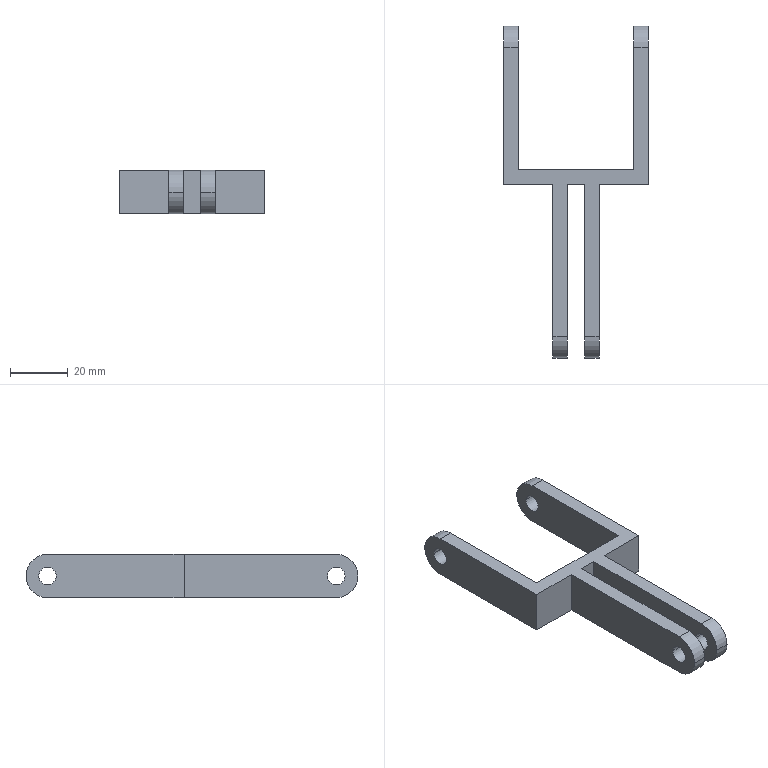Part | SolidWorks | features Extrusion 1, ICE 1 | 1 solid | 28 faces | box 50 x 115 x 15 mm | volume 19202 mm3 | cylinder 14 | plane 14 | commonest cylinder face diameters 6 x8 15 x6
STEP:
#1=CARTESIAN_POINT('',(8.,15.272,7.5));
#2=VERTEX_POINT('',#1);
#3=CARTESIAN_POINT('',(8.,9.272,7.5));
#4=VERTEX_POINT('',#3);
#5=CARTESIAN_POINT('',(8.,12.272,7.5));
#6=DIRECTION('',(-1.,0.,0.));
#7=DIRECTION('',(0.,-1.,0.));
#8=AXIS2_PLACEMENT_3D('',#5,#6,#7);
#9=CIRCLE('',#8,3.);
#10=EDGE_CURVE('',#2,#4,#9,.T.);
#11=ORIENTED_EDGE('',*,*,#10,.F.);
#12=CARTESIAN_POINT('',(3.,15.272,7.5));
#13=VERTEX_POINT('',#12);
#14=CARTESIAN_POINT('',(25.,15.272,7.5));
#15=DIRECTION('',(-1.,0.,0.));
#16=VECTOR('',#15,1000.);
#17=LINE('',#14,#16);
#18=EDGE_CURVE('',#2,#13,#17,.T.);
#19=ORIENTED_EDGE('',*,*,#18,.T.);
#20=CARTESIAN_POINT('',(3.,9.272,7.5));
#21=VERTEX_POINT('',#20);
#22=CARTESIAN_POINT('',(3.,12.272,7.5));
#23=DIRECTION('',(1.,0.,0.));
#24=DIRECTION('',(0.,1.,0.));
#25=AXIS2_PLACEMENT_3D('',#22,#23,#24);
#26=CIRCLE('',#25,3.);
#27=EDGE_CURVE('',#21,#13,#26,.T.);
#28=ORIENTED_EDGE('',*,*,#27,.F.);
#29=CARTESIAN_POINT('',(25.,9.272,7.5));
#30=DIRECTION('',(-1.,0.,0.));
#31=VECTOR('',#30,1000.);
#32=LINE('',#29,#31);
#33=EDGE_CURVE('',#4,#21,#32,.T.);
#34=ORIENTED_EDGE('',*,*,#33,.F.);
#35=EDGE_LOOP('',(#11,#19,#28,#34));
#36=FACE_OUTER_BOUND('',#35,.T.);
#37=CARTESIAN_POINT('',(25.,12.272,7.5));
#38=DIRECTION('',(-1.,0.,0.));
#39=DIRECTION('',(0.,-1.,0.));
#40=AXIS2_PLACEMENT_3D('',#37,#38,#39);
#41=CYLINDRICAL_SURFACE('',#40,3.);
#42=ADVANCED_FACE('',(#36),#41,.F.);
#43=CARTESIAN_POINT('',(25.,115.272,7.5));
#44=VERTEX_POINT('',#43);
#45=CARTESIAN_POINT('',(25.,109.272,7.5));
#46=VERTEX_POINT('',#45);
#47=CARTESIAN_POINT('',(25.,112.272,7.5));
#48=DIRECTION('',(-1.,0.,0.));
#49=DIRECTION('',(0.,-1.,0.));
#50=AXIS2_PLACEMENT_3D('',#47,#48,#49);
#51=CIRCLE('',#50,3.);
#52=EDGE_CURVE('',#44,#46,#51,.T.);
#53=ORIENTED_EDGE('',*,*,#52,.F.);
#54=CARTESIAN_POINT('',(20.,115.272,7.5));
#55=VERTEX_POINT('',#54);
#56=CARTESIAN_POINT('',(25.,115.272,7.5));
#57=DIRECTION('',(-1.,0.,0.));
#58=VECTOR('',#57,1000.);
#59=LINE('',#56,#58);
#60=EDGE_CURVE('',#44,#55,#59,.T.);
#61=ORIENTED_EDGE('',*,*,#60,.T.);
#62=CARTESIAN_POINT('',(20.,109.272,7.5));
#63=VERTEX_POINT('',#62);
#64=CARTESIAN_POINT('',(20.,112.272,7.5));
#65=DIRECTION('',(1.,0.,0.));
#66=DIRECTION('',(0.,0.,-1.));
#67=AXIS2_PLACEMENT_3D('',#64,#65,#66);
#68=CIRCLE('',#67,3.);
#69=EDGE_CURVE('',#63,#55,#68,.T.);
#70=ORIENTED_EDGE('',*,*,#69,.F.);
#71=CARTESIAN_POINT('',(25.,109.272,7.5));
#72=DIRECTION('',(-1.,0.,0.));
#73=VECTOR('',#72,1000.);
#74=LINE('',#71,#73);
#75=EDGE_CURVE('',#46,#63,#74,.T.);
#76=ORIENTED_EDGE('',*,*,#75,.F.);
#77=EDGE_LOOP('',(#53,#61,#70,#76));
#78=FACE_OUTER_BOUND('',#77,.T.);
#79=CARTESIAN_POINT('',(25.,112.272,7.5));
#80=DIRECTION('',(-1.,0.,0.));
#81=DIRECTION('',(0.,-1.,0.));
#82=AXIS2_PLACEMENT_3D('',#79,#80,#81);
#83=CYLINDRICAL_SURFACE('',#82,3.);
#84=ADVANCED_FACE('',(#78),#83,.F.);
#85=CARTESIAN_POINT('',(-20.,115.272,7.5));
#86=VERTEX_POINT('',#85);
#87=CARTESIAN_POINT('',(-20.,109.272,7.5));
#88=VERTEX_POINT('',#87);
#89=CARTESIAN_POINT('',(-20.,112.272,7.5));
#90=DIRECTION('',(-1.,0.,0.));
#91=DIRECTION('',(0.,0.,1.));
#92=AXIS2_PLACEMENT_3D('',#89,#90,#91);
#93=CIRCLE('',#92,3.);
#94=EDGE_CURVE('',#86,#88,#93,.T.);
#95=ORIENTED_EDGE('',*,*,#94,.F.);
#96=CARTESIAN_POINT('',(-25.,115.272,7.5));
#97=VERTEX_POINT('',#96);
#98=CARTESIAN_POINT('',(25.,115.272,7.5));
#99=DIRECTION('',(-1.,0.,0.));
#100=VECTOR('',#99,1000.);
#101=LINE('',#98,#100);
#102=EDGE_CURVE('',#86,#97,#101,.T.);
#103=ORIENTED_EDGE('',*,*,#102,.T.);
#104=CARTESIAN_POINT('',(-25.,109.272,7.5));
#105=VERTEX_POINT('',#104);
#106=CARTESIAN_POINT('',(-25.,112.272,7.5));
#107=DIRECTION('',(-1.,0.,0.));
#108=DIRECTION('',(0.,-1.,0.));
#109=AXIS2_PLACEMENT_3D('',#106,#107,#108);
#110=CIRCLE('',#109,3.);
#111=EDGE_CURVE('',#97,#105,#110,.T.);
#112=ORIENTED_EDGE('',*,*,#111,.T.);
#113=CARTESIAN_POINT('',(25.,109.272,7.5));
#114=DIRECTION('',(-1.,0.,0.));
#115=VECTOR('',#114,1000.);
#116=LINE('',#113,#115);
#117=EDGE_CURVE('',#88,#105,#116,.T.);
#118=ORIENTED_EDGE('',*,*,#117,.F.);
#119=EDGE_LOOP('',(#95,#103,#112,#118));
#120=FACE_OUTER_BOUND('',#119,.T.);
#121=CARTESIAN_POINT('',(25.,112.272,7.5));
#122=DIRECTION('',(-1.,0.,0.));
#123=DIRECTION('',(0.,-1.,0.));
#124=AXIS2_PLACEMENT_3D('',#121,#122,#123);
#125=CYLINDRICAL_SURFACE('',#124,3.);
#126=ADVANCED_FACE('',(#120),#125,.F.);
#127=CARTESIAN_POINT('',(-3.,15.272,7.5));
#128=VERTEX_POINT('',#127);
#129=CARTESIAN_POINT('',(-3.,9.272,7.5));
#130=VERTEX_POINT('',#129);
#131=CARTESIAN_POINT('',(-3.,12.272,7.5));
#132=DIRECTION('',(-1.,0.,0.));
#133=DIRECTION('',(0.,-1.,0.));
#134=AXIS2_PLACEMENT_3D('',#131,#132,#133);
#135=CIRCLE('',#134,3.);
#136=EDGE_CURVE('',#128,#130,#135,.T.);
#137=ORIENTED_EDGE('',*,*,#136,.F.);
#138=CARTESIAN_POINT('',(-8.,15.272,7.5));
#139=VERTEX_POINT('',#138);
#140=CARTESIAN_POINT('',(25.,15.272,7.5));
#141=DIRECTION('',(-1.,0.,0.));
#142=VECTOR('',#141,1000.);
#143=LINE('',#140,#142);
#144=EDGE_CURVE('',#128,#139,#143,.T.);
#145=ORIENTED_EDGE('',*,*,#144,.T.);
#146=CARTESIAN_POINT('',(-8.,9.272,7.5));
#147=VERTEX_POINT('',#146);
#148=CARTESIAN_POINT('',(-8.,12.272,7.5));
#149=DIRECTION('',(1.,0.,0.));
#150=DIRECTION('',(0.,1.,0.));
#151=AXIS2_PLACEMENT_3D('',#148,#149,#150);
#152=CIRCLE('',#151,3.);
#153=EDGE_CURVE('',#147,#139,#152,.T.);
#154=ORIENTED_EDGE('',*,*,#153,.F.);
#155=CARTESIAN_POINT('',(25.,9.272,7.5));
#156=DIRECTION('',(-1.,0.,0.));
#157=VECTOR('',#156,1000.);
#158=LINE('',#155,#157);
#159=EDGE_CURVE('',#130,#147,#158,.T.);
#160=ORIENTED_EDGE('',*,*,#159,.F.);
#161=EDGE_LOOP('',(#137,#145,#154,#160));
#162=FACE_OUTER_BOUND('',#161,.T.);
#163=CARTESIAN_POINT('',(25.,12.272,7.5));
#164=DIRECTION('',(-1.,0.,0.));
#165=DIRECTION('',(0.,-1.,0.));
#166=AXIS2_PLACEMENT_3D('',#163,#164,#165);
#167=CYLINDRICAL_SURFACE('',#166,3.);
#168=ADVANCED_FACE('',(#162),#167,.F.);
#169=CARTESIAN_POINT('',(8.,4.772,7.5));
#170=VERTEX_POINT('',#169);
#171=CARTESIAN_POINT('',(8.,12.272,0.));
#172=VERTEX_POINT('',#171);
#173=CARTESIAN_POINT('',(8.,12.272,7.5));
#174=DIRECTION('',(1.,0.,0.));
#175=DIRECTION('',(0.,-1.,0.));
#176=AXIS2_PLACEMENT_3D('',#173,#174,#175);
#177=CIRCLE('',#176,7.5);
#178=EDGE_CURVE('',#170,#172,#177,.T.);
#179=ORIENTED_EDGE('',*,*,#178,.F.);
#180=CARTESIAN_POINT('',(3.,4.772,7.5));
#181=VERTEX_POINT('',#180);
#182=CARTESIAN_POINT('',(25.,4.772,7.5));
#183=DIRECTION('',(-1.,0.,0.));
#184=VECTOR('',#183,1000.);
#185=LINE('',#182,#184);
#186=EDGE_CURVE('',#170,#181,#185,.T.);
#187=ORIENTED_EDGE('',*,*,#186,.T.);
#188=CARTESIAN_POINT('',(3.,12.272,0.));
#189=VERTEX_POINT('',#188);
#190=CARTESIAN_POINT('',(3.,12.272,7.5));
#191=DIRECTION('',(-1.,0.,0.));
#192=DIRECTION('',(0.,1.,0.));
#193=AXIS2_PLACEMENT_3D('',#190,#191,#192);
#194=CIRCLE('',#193,7.5);
#195=EDGE_CURVE('',#189,#181,#194,.T.);
#196=ORIENTED_EDGE('',*,*,#195,.F.);
#197=CARTESIAN_POINT('',(0.,12.272,0.));
#198=DIRECTION('',(-1.,0.,0.));
#199=VECTOR('',#198,1000.);
#200=LINE('',#197,#199);
#201=EDGE_CURVE('',#172,#189,#200,.T.);
#202=ORIENTED_EDGE('',*,*,#201,.F.);
#203=EDGE_LOOP('',(#179,#187,#196,#202));
#204=FACE_OUTER_BOUND('',#203,.T.);
#205=CARTESIAN_POINT('',(25.,12.272,7.5));
#206=DIRECTION('',(-1.,0.,0.));
#207=DIRECTION('',(0.,-1.,0.));
#208=AXIS2_PLACEMENT_3D('',#205,#206,#207);
#209=CYLINDRICAL_SURFACE('',#208,7.5);
#210=ADVANCED_FACE('',(#204),#209,.T.);
#211=CARTESIAN_POINT('',(-3.,4.772,7.5));
#212=VERTEX_POINT('',#211);
#213=CARTESIAN_POINT('',(-3.,12.272,0.));
#214=VERTEX_POINT('',#213);
#215=CARTESIAN_POINT('',(-3.,12.272,7.5));
#216=DIRECTION('',(1.,0.,0.));
#217=DIRECTION('',(0.,-1.,0.));
#218=AXIS2_PLACEMENT_3D('',#215,#216,#217);
#219=CIRCLE('',#218,7.5);
#220=EDGE_CURVE('',#212,#214,#219,.T.);
#221=ORIENTED_EDGE('',*,*,#220,.F.);
#222=CARTESIAN_POINT('',(-8.,4.772,7.5));
#223=VERTEX_POINT('',#222);
#224=CARTESIAN_POINT('',(25.,4.772,7.5));
#225=DIRECTION('',(-1.,0.,0.));
#226=VECTOR('',#225,1000.);
#227=LINE('',#224,#226);
#228=EDGE_CURVE('',#212,#223,#227,.T.);
#229=ORIENTED_EDGE('',*,*,#228,.T.);
#230=CARTESIAN_POINT('',(-8.,12.272,0.));
#231=VERTEX_POINT('',#230);
#232=CARTESIAN_POINT('',(-8.,12.272,7.5));
#233=DIRECTION('',(-1.,0.,0.));
#234=DIRECTION('',(0.,1.,0.));
#235=AXIS2_PLACEMENT_3D('',#232,#233,#234);
#236=CIRCLE('',#235,7.5);
#237=EDGE_CURVE('',#231,#223,#236,.T.);
#238=ORIENTED_EDGE('',*,*,#237,.F.);
#239=CARTESIAN_POINT('',(0.,12.272,0.));
#240=DIRECTION('',(-1.,0.,0.));
#241=VECTOR('',#240,1000.);
#242=LINE('',#239,#241);
#243=EDGE_CURVE('',#214,#231,#242,.T.);
#244=ORIENTED_EDGE('',*,*,#243,.F.);
#245=EDGE_LOOP('',(#221,#229,#238,#244));
#246=FACE_OUTER_BOUND('',#245,.T.);
#247=CARTESIAN_POINT('',(25.,12.272,7.5));
#248=DIRECTION('',(-1.,0.,0.));
#249=DIRECTION('',(0.,-1.,0.));
#250=AXIS2_PLACEMENT_3D('',#247,#248,#249);
#251=CYLINDRICAL_SURFACE('',#250,7.5);
#252=ADVANCED_FACE('',(#246),#251,.T.);
#253=CARTESIAN_POINT('',(-3.,12.272,15.));
#254=VERTEX_POINT('',#253);
#255=CARTESIAN_POINT('',(-3.,65.,15.));
#256=VERTEX_POINT('',#255);
#257=CARTESIAN_POINT('',(-3.,0.,15.));
#258=DIRECTION('',(0.,1.,0.));
#259=VECTOR('',#258,1000.);
#260=LINE('',#257,#259);
#261=EDGE_CURVE('',#254,#256,#260,.T.);
#262=ORIENTED_EDGE('',*,*,#261,.F.);
#263=CARTESIAN_POINT('',(-3.,12.272,7.5));
#264=DIRECTION('',(1.,0.,0.));
#265=DIRECTION('',(0.,-1.,0.));
#266=AXIS2_PLACEMENT_3D('',#263,#264,#265);
#267=CIRCLE('',#266,7.5);
#268=EDGE_CURVE('',#254,#212,#267,.T.);
#269=ORIENTED_EDGE('',*,*,#268,.T.);
#270=ORIENTED_EDGE('',*,*,#220,.T.);
#271=CARTESIAN_POINT('',(-3.,65.,0.));
#272=VERTEX_POINT('',#271);
#273=CARTESIAN_POINT('',(-3.,0.,0.));
#274=DIRECTION('',(0.,1.,0.));
#275=VECTOR('',#274,1000.);
#276=LINE('',#273,#275);
#277=EDGE_CURVE('',#214,#272,#276,.T.);
#278=ORIENTED_EDGE('',*,*,#277,.T.);
#279=CARTESIAN_POINT('',(-3.,65.,15.));
#280=DIRECTION('',(0.,0.,-1.));
#281=VECTOR('',#280,1000.);
#282=LINE('',#279,#281);
#283=EDGE_CURVE('',#256,#272,#282,.T.);
#284=ORIENTED_EDGE('',*,*,#283,.F.);
#285=EDGE_LOOP('',(#262,#269,#270,#278,#284));
#286=FACE_OUTER_BOUND('',#285,.T.);
#287=CARTESIAN_POINT('',(-3.,12.272,7.5));
#288=DIRECTION('',(-1.,0.,0.));
#289=DIRECTION('',(0.,-1.,0.));
#290=AXIS2_PLACEMENT_3D('',#287,#288,#289);
#291=CIRCLE('',#290,3.);
#292=EDGE_CURVE('',#130,#128,#291,.T.);
#293=ORIENTED_EDGE('',*,*,#292,.T.);
#294=ORIENTED_EDGE('',*,*,#136,.T.);
#295=EDGE_LOOP('',(#293,#294));
#296=FACE_BOUND('',#295,.T.);
#297=CARTESIAN_POINT('',(-3.,0.,15.));
#298=DIRECTION('',(-1.,0.,0.));
#299=DIRECTION('',(0.,-1.,0.));
#300=AXIS2_PLACEMENT_3D('',#297,#298,#299);
#301=PLANE('',#300);
#302=ADVANCED_FACE('',(#286,#296),#301,.F.);
#303=CARTESIAN_POINT('',(3.,65.,0.));
#304=VERTEX_POINT('',#303);
#305=CARTESIAN_POINT('',(3.,0.,0.));
#306=DIRECTION('',(0.,-1.,0.));
#307=VECTOR('',#306,1000.);
#308=LINE('',#305,#307);
#309=EDGE_CURVE('',#304,#189,#308,.T.);
#310=ORIENTED_EDGE('',*,*,#309,.T.);
#311=ORIENTED_EDGE('',*,*,#195,.T.);
#312=CARTESIAN_POINT('',(3.,12.272,15.));
#313=VERTEX_POINT('',#312);
#314=CARTESIAN_POINT('',(3.,12.272,7.5));
#315=DIRECTION('',(-1.,0.,0.));
#316=DIRECTION('',(0.,1.,0.));
#317=AXIS2_PLACEMENT_3D('',#314,#315,#316);
#318=CIRCLE('',#317,7.5);
#319=EDGE_CURVE('',#181,#313,#318,.T.);
#320=ORIENTED_EDGE('',*,*,#319,.T.);
#321=CARTESIAN_POINT('',(3.,65.,15.));
#322=VERTEX_POINT('',#321);
#323=CARTESIAN_POINT('',(3.,0.,15.));
#324=DIRECTION('',(0.,-1.,0.));
#325=VECTOR('',#324,1000.);
#326=LINE('',#323,#325);
#327=EDGE_CURVE('',#322,#313,#326,.T.);
#328=ORIENTED_EDGE('',*,*,#327,.F.);
#329=CARTESIAN_POINT('',(3.,65.,15.));
#330=DIRECTION('',(0.,0.,-1.));
#331=VECTOR('',#330,1000.);
#332=LINE('',#329,#331);
#333=EDGE_CURVE('',#322,#304,#332,.T.);
#334=ORIENTED_EDGE('',*,*,#333,.T.);
#335=EDGE_LOOP('',(#310,#311,#320,#328,#334));
#336=FACE_OUTER_BOUND('',#335,.T.);
#337=ORIENTED_EDGE('',*,*,#27,.T.);
#338=CARTESIAN_POINT('',(3.,12.272,7.5));
#339=DIRECTION('',(1.,0.,0.));
#340=DIRECTION('',(0.,1.,0.));
#341=AXIS2_PLACEMENT_3D('',#338,#339,#340);
#342=CIRCLE('',#341,3.);
#343=EDGE_CURVE('',#13,#21,#342,.T.);
#344=ORIENTED_EDGE('',*,*,#343,.T.);
#345=EDGE_LOOP('',(#337,#344));
#346=FACE_BOUND('',#345,.T.);
#347=CARTESIAN_POINT('',(3.,0.,15.));
#348=DIRECTION('',(1.,0.,0.));
#349=DIRECTION('',(0.,1.,0.));
#350=AXIS2_PLACEMENT_3D('',#347,#348,#349);
#351=PLANE('',#350);
#352=ADVANCED_FACE('',(#336,#346),#351,.F.);
#353=CARTESIAN_POINT('',(8.,12.272,15.));
#354=VERTEX_POINT('',#353);
#355=CARTESIAN_POINT('',(8.,65.,15.));
#356=VERTEX_POINT('',#355);
#357=CARTESIAN_POINT('',(8.,65.,15.));
#358=DIRECTION('',(0.,1.,0.));
#359=VECTOR('',#358,1000.);
#360=LINE('',#357,#359);
#361=EDGE_CURVE('',#354,#356,#360,.T.);
#362=ORIENTED_EDGE('',*,*,#361,.F.);
#363=CARTESIAN_POINT('',(8.,12.272,7.5));
#364=DIRECTION('',(1.,0.,0.));
#365=DIRECTION('',(0.,-1.,0.));
#366=AXIS2_PLACEMENT_3D('',#363,#364,#365);
#367=CIRCLE('',#366,7.5);
#368=EDGE_CURVE('',#354,#170,#367,.T.);
#369=ORIENTED_EDGE('',*,*,#368,.T.);
#370=ORIENTED_EDGE('',*,*,#178,.T.);
#371=CARTESIAN_POINT('',(8.,65.,0.));
#372=VERTEX_POINT('',#371);
#373=CARTESIAN_POINT('',(8.,65.,0.));
#374=DIRECTION('',(0.,1.,0.));
#375=VECTOR('',#374,1000.);
#376=LINE('',#373,#375);
#377=EDGE_CURVE('',#172,#372,#376,.T.);
#378=ORIENTED_EDGE('',*,*,#377,.T.);
#379=CARTESIAN_POINT('',(8.,65.,15.));
#380=DIRECTION('',(0.,0.,-1.));
#381=VECTOR('',#380,1000.);
#382=LINE('',#379,#381);
#383=EDGE_CURVE('',#356,#372,#382,.T.);
#384=ORIENTED_EDGE('',*,*,#383,.F.);
#385=EDGE_LOOP('',(#362,#369,#370,#378,#384));
#386=FACE_OUTER_BOUND('',#385,.T.);
#387=CARTESIAN_POINT('',(8.,12.272,7.5));
#388=DIRECTION('',(-1.,0.,0.));
#389=DIRECTION('',(0.,-1.,0.));
#390=AXIS2_PLACEMENT_3D('',#387,#388,#389);
#391=CIRCLE('',#390,3.);
#392=EDGE_CURVE('',#4,#2,#391,.T.);
#393=ORIENTED_EDGE('',*,*,#392,.T.);
#394=ORIENTED_EDGE('',*,*,#10,.T.);
#395=EDGE_LOOP('',(#393,#394));
#396=FACE_BOUND('',#395,.T.);
#397=CARTESIAN_POINT('',(8.,65.,15.));
#398=DIRECTION('',(-1.,0.,0.));
#399=DIRECTION('',(0.,-1.,0.));
#400=AXIS2_PLACEMENT_3D('',#397,#398,#399);
#401=PLANE('',#400);
#402=ADVANCED_FACE('',(#386,#396),#401,.F.);
#403=CARTESIAN_POINT('',(-8.,65.,0.));
#404=VERTEX_POINT('',#403);
#405=CARTESIAN_POINT('',(-8.,65.,0.));
#406=DIRECTION('',(0.,-1.,0.));
#407=VECTOR('',#406,1000.);
#408=LINE('',#405,#407);
#409=EDGE_CURVE('',#404,#231,#408,.T.);
#410=ORIENTED_EDGE('',*,*,#409,.T.);
#411=ORIENTED_EDGE('',*,*,#237,.T.);
#412=CARTESIAN_POINT('',(-8.,12.272,15.));
#413=VERTEX_POINT('',#412);
#414=CARTESIAN_POINT('',(-8.,12.272,7.5));
#415=DIRECTION('',(-1.,0.,0.));
#416=DIRECTION('',(0.,1.,0.));
#417=AXIS2_PLACEMENT_3D('',#414,#415,#416);
#418=CIRCLE('',#417,7.5);
#419=EDGE_CURVE('',#223,#413,#418,.T.);
#420=ORIENTED_EDGE('',*,*,#419,.T.);
#421=CARTESIAN_POINT('',(-8.,65.,15.));
#422=VERTEX_POINT('',#421);
#423=CARTESIAN_POINT('',(-8.,65.,15.));
#424=DIRECTION('',(0.,-1.,0.));
#425=VECTOR('',#424,1000.);
#426=LINE('',#423,#425);
#427=EDGE_CURVE('',#422,#413,#426,.T.);
#428=ORIENTED_EDGE('',*,*,#427,.F.);
#429=CARTESIAN_POINT('',(-8.,65.,15.));
#430=DIRECTION('',(0.,0.,-1.));
#431=VECTOR('',#430,1000.);
#432=LINE('',#429,#431);
#433=EDGE_CURVE('',#422,#404,#432,.T.);
#434=ORIENTED_EDGE('',*,*,#433,.T.);
#435=EDGE_LOOP('',(#410,#411,#420,#428,#434));
#436=FACE_OUTER_BOUND('',#435,.T.);
#437=ORIENTED_EDGE('',*,*,#153,.T.);
#438=CARTESIAN_POINT('',(-8.,12.272,7.5));
#439=DIRECTION('',(1.,0.,0.));
#440=DIRECTION('',(0.,1.,0.));
#441=AXIS2_PLACEMENT_3D('',#438,#439,#440);
#442=CIRCLE('',#441,3.);
#443=EDGE_CURVE('',#139,#147,#442,.T.);
#444=ORIENTED_EDGE('',*,*,#443,.T.);
#445=EDGE_LOOP('',(#437,#444));
#446=FACE_BOUND('',#445,.T.);
#447=CARTESIAN_POINT('',(-8.,65.,15.));
#448=DIRECTION('',(1.,0.,0.));
#449=DIRECTION('',(0.,1.,0.));
#450=AXIS2_PLACEMENT_3D('',#447,#448,#449);
#451=PLANE('',#450);
#452=ADVANCED_FACE('',(#436,#446),#451,.F.);
#453=CARTESIAN_POINT('',(-3.,65.,0.));
#454=DIRECTION('',(1.,0.,0.));
#455=VECTOR('',#454,1000.);
#456=LINE('',#453,#455);
#457=EDGE_CURVE('',#272,#304,#456,.T.);
#458=ORIENTED_EDGE('',*,*,#457,.T.);
#459=ORIENTED_EDGE('',*,*,#333,.F.);
#460=CARTESIAN_POINT('',(-3.,65.,15.));
#461=DIRECTION('',(1.,0.,0.));
#462=VECTOR('',#461,1000.);
#463=LINE('',#460,#462);
#464=EDGE_CURVE('',#256,#322,#463,.T.);
#465=ORIENTED_EDGE('',*,*,#464,.F.);
#466=ORIENTED_EDGE('',*,*,#283,.T.);
#467=EDGE_LOOP('',(#458,#459,#465,#466));
#468=FACE_OUTER_BOUND('',#467,.T.);
#469=CARTESIAN_POINT('',(-3.,65.,15.));
#470=DIRECTION('',(0.,1.,0.));
#471=DIRECTION('',(0.,0.,1.));
#472=AXIS2_PLACEMENT_3D('',#469,#470,#471);
#473=PLANE('',#472);
#474=ADVANCED_FACE('',(#468),#473,.F.);
#475=CARTESIAN_POINT('',(25.,65.,0.));
#476=VERTEX_POINT('',#475);
#477=CARTESIAN_POINT('',(25.,65.,0.));
#478=DIRECTION('',(1.,0.,0.));
#479=VECTOR('',#478,1000.);
#480=LINE('',#477,#479);
#481=EDGE_CURVE('',#372,#476,#480,.T.);
#482=ORIENTED_EDGE('',*,*,#481,.T.);
#483=CARTESIAN_POINT('',(25.,65.,15.));
#484=VERTEX_POINT('',#483);
#485=CARTESIAN_POINT('',(25.,65.,15.));
#486=DIRECTION('',(0.,0.,-1.));
#487=VECTOR('',#486,1000.);
#488=LINE('',#485,#487);
#489=EDGE_CURVE('',#484,#476,#488,.T.);
#490=ORIENTED_EDGE('',*,*,#489,.F.);
#491=CARTESIAN_POINT('',(25.,65.,15.));
#492=DIRECTION('',(1.,0.,0.));
#493=VECTOR('',#492,1000.);
#494=LINE('',#491,#493);
#495=EDGE_CURVE('',#356,#484,#494,.T.);
#496=ORIENTED_EDGE('',*,*,#495,.F.);
#497=ORIENTED_EDGE('',*,*,#383,.T.);
#498=EDGE_LOOP('',(#482,#490,#496,#497));
#499=FACE_OUTER_BOUND('',#498,.T.);
#500=CARTESIAN_POINT('',(25.,65.,15.));
#501=DIRECTION('',(0.,1.,0.));
#502=DIRECTION('',(0.,0.,1.));
#503=AXIS2_PLACEMENT_3D('',#500,#501,#502);
#504=PLANE('',#503);
#505=ADVANCED_FACE('',(#499),#504,.F.);
#506=CARTESIAN_POINT('',(25.,112.272,7.5));
#507=DIRECTION('',(-1.,0.,0.));
#508=DIRECTION('',(0.,-1.,0.));
#509=AXIS2_PLACEMENT_3D('',#506,#507,#508);
#510=CIRCLE('',#509,3.);
#511=EDGE_CURVE('',#46,#44,#510,.T.);
#512=ORIENTED_EDGE('',*,*,#511,.T.);
#513=ORIENTED_EDGE('',*,*,#52,.T.);
#514=EDGE_LOOP('',(#512,#513));
#515=FACE_BOUND('',#514,.T.);
#516=CARTESIAN_POINT('',(25.,112.272,0.));
#517=VERTEX_POINT('',#516);
#518=CARTESIAN_POINT('',(25.,120.,0.));
#519=DIRECTION('',(0.,1.,0.));
#520=VECTOR('',#519,1000.);
#521=LINE('',#518,#520);
#522=EDGE_CURVE('',#476,#517,#521,.T.);
#523=ORIENTED_EDGE('',*,*,#522,.T.);
#524=CARTESIAN_POINT('',(25.,112.272,15.));
#525=VERTEX_POINT('',#524);
#526=CARTESIAN_POINT('',(25.,112.272,7.5));
#527=DIRECTION('',(1.,0.,0.));
#528=DIRECTION('',(0.,-1.,0.));
#529=AXIS2_PLACEMENT_3D('',#526,#527,#528);
#530=CIRCLE('',#529,7.5);
#531=EDGE_CURVE('',#517,#525,#530,.T.);
#532=ORIENTED_EDGE('',*,*,#531,.T.);
#533=CARTESIAN_POINT('',(25.,120.,15.));
#534=DIRECTION('',(0.,1.,0.));
#535=VECTOR('',#534,1000.);
#536=LINE('',#533,#535);
#537=EDGE_CURVE('',#484,#525,#536,.T.);
#538=ORIENTED_EDGE('',*,*,#537,.F.);
#539=ORIENTED_EDGE('',*,*,#489,.T.);
#540=EDGE_LOOP('',(#523,#532,#538,#539));
#541=FACE_OUTER_BOUND('',#540,.T.);
#542=CARTESIAN_POINT('',(25.,120.,15.));
#543=DIRECTION('',(-1.,0.,0.));
#544=DIRECTION('',(0.,-1.,0.));
#545=AXIS2_PLACEMENT_3D('',#542,#543,#544);
#546=PLANE('',#545);
#547=ADVANCED_FACE('',(#515,#541),#546,.F.);
#548=ORIENTED_EDGE('',*,*,#69,.T.);
#549=CARTESIAN_POINT('',(20.,112.272,7.5));
#550=DIRECTION('',(1.,0.,0.));
#551=DIRECTION('',(0.,0.,-1.));
#552=AXIS2_PLACEMENT_3D('',#549,#550,#551);
#553=CIRCLE('',#552,3.);
#554=EDGE_CURVE('',#55,#63,#553,.T.);
#555=ORIENTED_EDGE('',*,*,#554,.T.);
#556=EDGE_LOOP('',(#548,#555));
#557=FACE_BOUND('',#556,.T.);
#558=CARTESIAN_POINT('',(20.,112.272,15.));
#559=VERTEX_POINT('',#558);
#560=CARTESIAN_POINT('',(20.,70.,15.));
#561=VERTEX_POINT('',#560);
#562=CARTESIAN_POINT('',(20.,70.,15.));
#563=DIRECTION('',(0.,-1.,0.));
#564=VECTOR('',#563,1000.);
#565=LINE('',#562,#564);
#566=EDGE_CURVE('',#559,#561,#565,.T.);
#567=ORIENTED_EDGE('',*,*,#566,.F.);
#568=CARTESIAN_POINT('',(20.,112.272,0.));
#569=VERTEX_POINT('',#568);
#570=CARTESIAN_POINT('',(20.,112.272,7.5));
#571=DIRECTION('',(-1.,0.,0.));
#572=DIRECTION('',(0.,0.,-1.));
#573=AXIS2_PLACEMENT_3D('',#570,#571,#572);
#574=CIRCLE('',#573,7.5);
#575=EDGE_CURVE('',#559,#569,#574,.T.);
#576=ORIENTED_EDGE('',*,*,#575,.T.);
#577=CARTESIAN_POINT('',(20.,70.,0.));
#578=VERTEX_POINT('',#577);
#579=CARTESIAN_POINT('',(20.,70.,0.));
#580=DIRECTION('',(0.,-1.,0.));
#581=VECTOR('',#580,1000.);
#582=LINE('',#579,#581);
#583=EDGE_CURVE('',#569,#578,#582,.T.);
#584=ORIENTED_EDGE('',*,*,#583,.T.);
#585=CARTESIAN_POINT('',(20.,70.,15.));
#586=DIRECTION('',(0.,0.,-1.));
#587=VECTOR('',#586,1000.);
#588=LINE('',#585,#587);
#589=EDGE_CURVE('',#561,#578,#588,.T.);
#590=ORIENTED_EDGE('',*,*,#589,.F.);
#591=EDGE_LOOP('',(#567,#576,#584,#590));
#592=FACE_OUTER_BOUND('',#591,.T.);
#593=CARTESIAN_POINT('',(20.,70.,15.));
#594=DIRECTION('',(1.,0.,0.));
#595=DIRECTION('',(0.,0.,-1.));
#596=AXIS2_PLACEMENT_3D('',#593,#594,#595);
#597=PLANE('',#596);
#598=ADVANCED_FACE('',(#557,#592),#597,.F.);
#599=CARTESIAN_POINT('',(-20.,70.,0.));
#600=VERTEX_POINT('',#599);
#601=CARTESIAN_POINT('',(20.,70.,0.));
#602=DIRECTION('',(-1.,0.,0.));
#603=VECTOR('',#602,1000.);
#604=LINE('',#601,#603);
#605=EDGE_CURVE('',#578,#600,#604,.T.);
#606=ORIENTED_EDGE('',*,*,#605,.T.);
#607=CARTESIAN_POINT('',(-20.,70.,15.));
#608=VERTEX_POINT('',#607);
#609=CARTESIAN_POINT('',(-20.,70.,15.));
#610=DIRECTION('',(0.,0.,-1.));
#611=VECTOR('',#610,1000.);
#612=LINE('',#609,#611);
#613=EDGE_CURVE('',#608,#600,#612,.T.);
#614=ORIENTED_EDGE('',*,*,#613,.F.);
#615=CARTESIAN_POINT('',(20.,70.,15.));
#616=DIRECTION('',(-1.,0.,0.));
#617=VECTOR('',#616,1000.);
#618=LINE('',#615,#617);
#619=EDGE_CURVE('',#561,#608,#618,.T.);
#620=ORIENTED_EDGE('',*,*,#619,.F.);
#621=ORIENTED_EDGE('',*,*,#589,.T.);
#622=EDGE_LOOP('',(#606,#614,#620,#621));
#623=FACE_OUTER_BOUND('',#622,.T.);
#624=CARTESIAN_POINT('',(20.,70.,15.));
#625=DIRECTION('',(0.,-1.,0.));
#626=DIRECTION('',(0.,0.,-1.));
#627=AXIS2_PLACEMENT_3D('',#624,#625,#626);
#628=PLANE('',#627);
#629=ADVANCED_FACE('',(#623),#628,.F.);
#630=CARTESIAN_POINT('',(-20.,112.272,7.5));
#631=DIRECTION('',(-1.,0.,0.));
#632=DIRECTION('',(0.,0.,1.));
#633=AXIS2_PLACEMENT_3D('',#630,#631,#632);
#634=CIRCLE('',#633,3.);
#635=EDGE_CURVE('',#88,#86,#634,.T.);
#636=ORIENTED_EDGE('',*,*,#635,.T.);
#637=ORIENTED_EDGE('',*,*,#94,.T.);
#638=EDGE_LOOP('',(#636,#637));
#639=FACE_BOUND('',#638,.T.);
#640=CARTESIAN_POINT('',(-20.,112.272,0.));
#641=VERTEX_POINT('',#640);
#642=CARTESIAN_POINT('',(-20.,70.,0.));
#643=DIRECTION('',(0.,1.,0.));
#644=VECTOR('',#643,1000.);
#645=LINE('',#642,#644);
#646=EDGE_CURVE('',#600,#641,#645,.T.);
#647=ORIENTED_EDGE('',*,*,#646,.T.);
#648=CARTESIAN_POINT('',(-20.,112.272,15.));
#649=VERTEX_POINT('',#648);
#650=CARTESIAN_POINT('',(-20.,112.272,7.5));
#651=DIRECTION('',(1.,0.,0.));
#652=DIRECTION('',(0.,0.,1.));
#653=AXIS2_PLACEMENT_3D('',#650,#651,#652);
#654=CIRCLE('',#653,7.5);
#655=EDGE_CURVE('',#641,#649,#654,.T.);
#656=ORIENTED_EDGE('',*,*,#655,.T.);
#657=CARTESIAN_POINT('',(-20.,70.,15.));
#658=DIRECTION('',(0.,1.,0.));
#659=VECTOR('',#658,1000.);
#660=LINE('',#657,#659);
#661=EDGE_CURVE('',#608,#649,#660,.T.);
#662=ORIENTED_EDGE('',*,*,#661,.F.);
#663=ORIENTED_EDGE('',*,*,#613,.T.);
#664=EDGE_LOOP('',(#647,#656,#662,#663));
#665=FACE_OUTER_BOUND('',#664,.T.);
#666=CARTESIAN_POINT('',(-20.,70.,15.));
#667=DIRECTION('',(-1.,0.,0.));
#668=DIRECTION('',(0.,0.,1.));
#669=AXIS2_PLACEMENT_3D('',#666,#667,#668);
#670=PLANE('',#669);
#671=ADVANCED_FACE('',(#639,#665),#670,.F.);
#672=CARTESIAN_POINT('',(-25.,112.272,7.5));
#673=DIRECTION('',(-1.,0.,0.));
#674=DIRECTION('',(0.,-1.,0.));
#675=AXIS2_PLACEMENT_3D('',#672,#673,#674);
#676=CIRCLE('',#675,3.);
#677=EDGE_CURVE('',#105,#97,#676,.T.);
#678=ORIENTED_EDGE('',*,*,#677,.F.);
#679=ORIENTED_EDGE('',*,*,#111,.F.);
#680=EDGE_LOOP('',(#678,#679));
#681=FACE_BOUND('',#680,.T.);
#682=CARTESIAN_POINT('',(-25.,112.272,15.));
#683=VERTEX_POINT('',#682);
#684=CARTESIAN_POINT('',(-25.,65.,15.));
#685=VERTEX_POINT('',#684);
#686=CARTESIAN_POINT('',(-25.,120.,15.));
#687=DIRECTION('',(0.,-1.,0.));
#688=VECTOR('',#687,1000.);
#689=LINE('',#686,#688);
#690=EDGE_CURVE('',#683,#685,#689,.T.);
#691=ORIENTED_EDGE('',*,*,#690,.F.);
#692=CARTESIAN_POINT('',(-25.,112.272,0.));
#693=VERTEX_POINT('',#692);
#694=CARTESIAN_POINT('',(-25.,112.272,7.5));
#695=DIRECTION('',(1.,0.,0.));
#696=DIRECTION('',(0.,-1.,0.));
#697=AXIS2_PLACEMENT_3D('',#694,#695,#696);
#698=CIRCLE('',#697,7.5);
#699=EDGE_CURVE('',#693,#683,#698,.T.);
#700=ORIENTED_EDGE('',*,*,#699,.F.);
#701=CARTESIAN_POINT('',(-25.,65.,0.));
#702=VERTEX_POINT('',#701);
#703=CARTESIAN_POINT('',(-25.,120.,0.));
#704=DIRECTION('',(0.,-1.,0.));
#705=VECTOR('',#704,1000.);
#706=LINE('',#703,#705);
#707=EDGE_CURVE('',#693,#702,#706,.T.);
#708=ORIENTED_EDGE('',*,*,#707,.T.);
#709=CARTESIAN_POINT('',(-25.,65.,15.));
#710=DIRECTION('',(0.,0.,-1.));
#711=VECTOR('',#710,1000.);
#712=LINE('',#709,#711);
#713=EDGE_CURVE('',#685,#702,#712,.T.);
#714=ORIENTED_EDGE('',*,*,#713,.F.);
#715=EDGE_LOOP('',(#691,#700,#708,#714));
#716=FACE_OUTER_BOUND('',#715,.T.);
#717=CARTESIAN_POINT('',(-25.,120.,15.));
#718=DIRECTION('',(1.,0.,0.));
#719=DIRECTION('',(0.,1.,0.));
#720=AXIS2_PLACEMENT_3D('',#717,#718,#719);
#721=PLANE('',#720);
#722=ADVANCED_FACE('',(#681,#716),#721,.F.);
#723=CARTESIAN_POINT('',(-25.,65.,0.));
#724=DIRECTION('',(1.,0.,0.));
#725=VECTOR('',#724,1000.);
#726=LINE('',#723,#725);
#727=EDGE_CURVE('',#702,#404,#726,.T.);
#728=ORIENTED_EDGE('',*,*,#727,.T.);
#729=ORIENTED_EDGE('',*,*,#433,.F.);
#730=CARTESIAN_POINT('',(-25.,65.,15.));
#731=DIRECTION('',(1.,0.,0.));
#732=VECTOR('',#731,1000.);
#733=LINE('',#730,#732);
#734=EDGE_CURVE('',#685,#422,#733,.T.);
#735=ORIENTED_EDGE('',*,*,#734,.F.);
#736=ORIENTED_EDGE('',*,*,#713,.T.);
#737=EDGE_LOOP('',(#728,#729,#735,#736));
#738=FACE_OUTER_BOUND('',#737,.T.);
#739=CARTESIAN_POINT('',(-25.,65.,15.));
#740=DIRECTION('',(0.,1.,0.));
#741=DIRECTION('',(0.,0.,1.));
#742=AXIS2_PLACEMENT_3D('',#739,#740,#741);
#743=PLANE('',#742);
#744=ADVANCED_FACE('',(#738),#743,.F.);
#745=CARTESIAN_POINT('',(25.,112.272,15.));
#746=DIRECTION('',(-1.,0.,0.));
#747=VECTOR('',#746,1000.);
#748=LINE('',#745,#747);
#749=EDGE_CURVE('',#649,#683,#748,.T.);
#750=ORIENTED_EDGE('',*,*,#749,.T.);
#751=ORIENTED_EDGE('',*,*,#690,.T.);
#752=ORIENTED_EDGE('',*,*,#734,.T.);
#753=ORIENTED_EDGE('',*,*,#427,.T.);
#754=CARTESIAN_POINT('',(25.,12.272,15.));
#755=DIRECTION('',(-1.,0.,0.));
#756=VECTOR('',#755,1000.);
#757=LINE('',#754,#756);
#758=EDGE_CURVE('',#254,#413,#757,.T.);
#759=ORIENTED_EDGE('',*,*,#758,.F.);
#760=ORIENTED_EDGE('',*,*,#261,.T.);
#761=ORIENTED_EDGE('',*,*,#464,.T.);
#762=ORIENTED_EDGE('',*,*,#327,.T.);
#763=CARTESIAN_POINT('',(25.,12.272,15.));
#764=DIRECTION('',(-1.,0.,0.));
#765=VECTOR('',#764,1000.);
#766=LINE('',#763,#765);
#767=EDGE_CURVE('',#354,#313,#766,.T.);
#768=ORIENTED_EDGE('',*,*,#767,.F.);
#769=ORIENTED_EDGE('',*,*,#361,.T.);
#770=ORIENTED_EDGE('',*,*,#495,.T.);
#771=ORIENTED_EDGE('',*,*,#537,.T.);
#772=CARTESIAN_POINT('',(25.,112.272,15.));
#773=DIRECTION('',(-1.,0.,0.));
#774=VECTOR('',#773,1000.);
#775=LINE('',#772,#774);
#776=EDGE_CURVE('',#525,#559,#775,.T.);
#777=ORIENTED_EDGE('',*,*,#776,.T.);
#778=ORIENTED_EDGE('',*,*,#566,.T.);
#779=ORIENTED_EDGE('',*,*,#619,.T.);
#780=ORIENTED_EDGE('',*,*,#661,.T.);
#781=EDGE_LOOP('',(#750,#751,#752,#753,#759,#760,#761,#762,#768,#769,#770,#771,#777,#778,#779,#780));
#782=FACE_OUTER_BOUND('',#781,.T.);
#783=CARTESIAN_POINT('',(0.,0.,15.));
#784=DIRECTION('',(0.,0.,1.));
#785=DIRECTION('',(1.,0.,0.));
#786=AXIS2_PLACEMENT_3D('',#783,#784,#785);
#787=PLANE('',#786);
#788=ADVANCED_FACE('',(#782),#787,.T.);
#789=ORIENTED_EDGE('',*,*,#707,.F.);
#790=CARTESIAN_POINT('',(0.,112.272,0.));
#791=DIRECTION('',(1.,0.,0.));
#792=VECTOR('',#791,1000.);
#793=LINE('',#790,#792);
#794=EDGE_CURVE('',#693,#641,#793,.T.);
#795=ORIENTED_EDGE('',*,*,#794,.T.);
#796=ORIENTED_EDGE('',*,*,#646,.F.);
#797=ORIENTED_EDGE('',*,*,#605,.F.);
#798=ORIENTED_EDGE('',*,*,#583,.F.);
#799=CARTESIAN_POINT('',(25.,112.272,0.));
#800=DIRECTION('',(-1.,0.,0.));
#801=VECTOR('',#800,1000.);
#802=LINE('',#799,#801);
#803=EDGE_CURVE('',#517,#569,#802,.T.);
#804=ORIENTED_EDGE('',*,*,#803,.F.);
#805=ORIENTED_EDGE('',*,*,#522,.F.);
#806=ORIENTED_EDGE('',*,*,#481,.F.);
#807=ORIENTED_EDGE('',*,*,#377,.F.);
#808=ORIENTED_EDGE('',*,*,#201,.T.);
#809=ORIENTED_EDGE('',*,*,#309,.F.);
#810=ORIENTED_EDGE('',*,*,#457,.F.);
#811=ORIENTED_EDGE('',*,*,#277,.F.);
#812=ORIENTED_EDGE('',*,*,#243,.T.);
#813=ORIENTED_EDGE('',*,*,#409,.F.);
#814=ORIENTED_EDGE('',*,*,#727,.F.);
#815=EDGE_LOOP('',(#789,#795,#796,#797,#798,#804,#805,#806,#807,#808,#809,#810,#811,#812,#813,#814));
#816=FACE_OUTER_BOUND('',#815,.T.);
#817=CARTESIAN_POINT('',(0.,0.,0.));
#818=DIRECTION('',(0.,0.,1.));
#819=DIRECTION('',(1.,0.,0.));
#820=AXIS2_PLACEMENT_3D('',#817,#818,#819);
#821=PLANE('',#820);
#822=ADVANCED_FACE('',(#816),#821,.F.);
#823=ORIENTED_EDGE('',*,*,#228,.F.);
#824=ORIENTED_EDGE('',*,*,#268,.F.);
#825=ORIENTED_EDGE('',*,*,#758,.T.);
#826=ORIENTED_EDGE('',*,*,#419,.F.);
#827=EDGE_LOOP('',(#823,#824,#825,#826));
#828=FACE_OUTER_BOUND('',#827,.T.);
#829=CARTESIAN_POINT('',(25.,12.272,7.5));
#830=DIRECTION('',(-1.,0.,0.));
#831=DIRECTION('',(0.,-1.,0.));
#832=AXIS2_PLACEMENT_3D('',#829,#830,#831);
#833=CYLINDRICAL_SURFACE('',#832,7.5);
#834=ADVANCED_FACE('',(#828),#833,.T.);
#835=ORIENTED_EDGE('',*,*,#186,.F.);
#836=ORIENTED_EDGE('',*,*,#368,.F.);
#837=ORIENTED_EDGE('',*,*,#767,.T.);
#838=ORIENTED_EDGE('',*,*,#319,.F.);
#839=EDGE_LOOP('',(#835,#836,#837,#838));
#840=FACE_OUTER_BOUND('',#839,.T.);
#841=CARTESIAN_POINT('',(25.,12.272,7.5));
#842=DIRECTION('',(-1.,0.,0.));
#843=DIRECTION('',(0.,-1.,0.));
#844=AXIS2_PLACEMENT_3D('',#841,#842,#843);
#845=CYLINDRICAL_SURFACE('',#844,7.5);
#846=ADVANCED_FACE('',(#840),#845,.T.);
#847=ORIENTED_EDGE('',*,*,#776,.F.);
#848=ORIENTED_EDGE('',*,*,#531,.F.);
#849=ORIENTED_EDGE('',*,*,#803,.T.);
#850=ORIENTED_EDGE('',*,*,#575,.F.);
#851=EDGE_LOOP('',(#847,#848,#849,#850));
#852=FACE_OUTER_BOUND('',#851,.T.);
#853=CARTESIAN_POINT('',(25.,112.272,7.5));
#854=DIRECTION('',(-1.,0.,0.));
#855=DIRECTION('',(0.,-1.,0.));
#856=AXIS2_PLACEMENT_3D('',#853,#854,#855);
#857=CYLINDRICAL_SURFACE('',#856,7.5);
#858=ADVANCED_FACE('',(#852),#857,.T.);
#859=ORIENTED_EDGE('',*,*,#794,.F.);
#860=ORIENTED_EDGE('',*,*,#699,.T.);
#861=ORIENTED_EDGE('',*,*,#749,.F.);
#862=ORIENTED_EDGE('',*,*,#655,.F.);
#863=EDGE_LOOP('',(#859,#860,#861,#862));
#864=FACE_OUTER_BOUND('',#863,.T.);
#865=CARTESIAN_POINT('',(25.,112.272,7.5));
#866=DIRECTION('',(-1.,0.,0.));
#867=DIRECTION('',(0.,-1.,0.));
#868=AXIS2_PLACEMENT_3D('',#865,#866,#867);
#869=CYLINDRICAL_SURFACE('',#868,7.5);
#870=ADVANCED_FACE('',(#864),#869,.T.);
#871=ORIENTED_EDGE('',*,*,#144,.F.);
#872=ORIENTED_EDGE('',*,*,#292,.F.);
#873=ORIENTED_EDGE('',*,*,#159,.T.);
#874=ORIENTED_EDGE('',*,*,#443,.F.);
#875=EDGE_LOOP('',(#871,#872,#873,#874));
#876=FACE_OUTER_BOUND('',#875,.T.);
#877=CARTESIAN_POINT('',(25.,12.272,7.5));
#878=DIRECTION('',(-1.,0.,0.));
#879=DIRECTION('',(0.,-1.,0.));
#880=AXIS2_PLACEMENT_3D('',#877,#878,#879);
#881=CYLINDRICAL_SURFACE('',#880,3.);
#882=ADVANCED_FACE('',(#876),#881,.F.);
#883=ORIENTED_EDGE('',*,*,#102,.F.);
#884=ORIENTED_EDGE('',*,*,#635,.F.);
#885=ORIENTED_EDGE('',*,*,#117,.T.);
#886=ORIENTED_EDGE('',*,*,#677,.T.);
#887=EDGE_LOOP('',(#883,#884,#885,#886));
#888=FACE_OUTER_BOUND('',#887,.T.);
#889=CARTESIAN_POINT('',(25.,112.272,7.5));
#890=DIRECTION('',(-1.,0.,0.));
#891=DIRECTION('',(0.,-1.,0.));
#892=AXIS2_PLACEMENT_3D('',#889,#890,#891);
#893=CYLINDRICAL_SURFACE('',#892,3.);
#894=ADVANCED_FACE('',(#888),#893,.F.);
#895=ORIENTED_EDGE('',*,*,#60,.F.);
#896=ORIENTED_EDGE('',*,*,#511,.F.);
#897=ORIENTED_EDGE('',*,*,#75,.T.);
#898=ORIENTED_EDGE('',*,*,#554,.F.);
#899=EDGE_LOOP('',(#895,#896,#897,#898));
#900=FACE_OUTER_BOUND('',#899,.T.);
#901=CARTESIAN_POINT('',(25.,112.272,7.5));
#902=DIRECTION('',(-1.,0.,0.));
#903=DIRECTION('',(0.,-1.,0.));
#904=AXIS2_PLACEMENT_3D('',#901,#902,#903);
#905=CYLINDRICAL_SURFACE('',#904,3.);
#906=ADVANCED_FACE('',(#900),#905,.F.);
#907=ORIENTED_EDGE('',*,*,#18,.F.);
#908=ORIENTED_EDGE('',*,*,#392,.F.);
#909=ORIENTED_EDGE('',*,*,#33,.T.);
#910=ORIENTED_EDGE('',*,*,#343,.F.);
#911=EDGE_LOOP('',(#907,#908,#909,#910));
#912=FACE_OUTER_BOUND('',#911,.T.);
#913=CARTESIAN_POINT('',(25.,12.272,7.5));
#914=DIRECTION('',(-1.,0.,0.));
#915=DIRECTION('',(0.,-1.,0.));
#916=AXIS2_PLACEMENT_3D('',#913,#914,#915);
#917=CYLINDRICAL_SURFACE('',#916,3.);
#918=ADVANCED_FACE('',(#912),#917,.F.);
#919=CLOSED_SHELL('',(#42,#84,#126,#168,#210,#252,#302,#352,#402,#452,#474,#505,#547,#598,#629,#671,#722,#744,#788,#822,#834,#846,#858,#870,#882,#894,#906,#918));
#920=MANIFOLD_SOLID_BREP('',#919);
#921=CARTESIAN_POINT('',(0.,0.,0.));
#922=DIRECTION('',(0.,0.,1.));
#923=DIRECTION('',(1.,0.,0.));
#924=AXIS2_PLACEMENT_3D('',#921,#922,#923);
#925=(LENGTH_UNIT()NAMED_UNIT(*)SI_UNIT(.MILLI.,.METRE.));
#926=UNCERTAINTY_MEASURE_WITH_UNIT(LENGTH_MEASURE(0.00001),#925,'','');
#927=(NAMED_UNIT(*)PLANE_ANGLE_UNIT()SI_UNIT($,.RADIAN.));
#928=(NAMED_UNIT(*)SI_UNIT($,.STERADIAN.)SOLID_ANGLE_UNIT());
#929=(GEOMETRIC_REPRESENTATION_CONTEXT(3)GLOBAL_UNCERTAINTY_ASSIGNED_CONTEXT((#926))GLOBAL_UNIT_ASSIGNED_CONTEXT((#925,#927,#928))REPRESENTATION_CONTEXT('',''));
#930=ADVANCED_BREP_SHAPE_REPRESENTATION('',(#920,#924),#929);